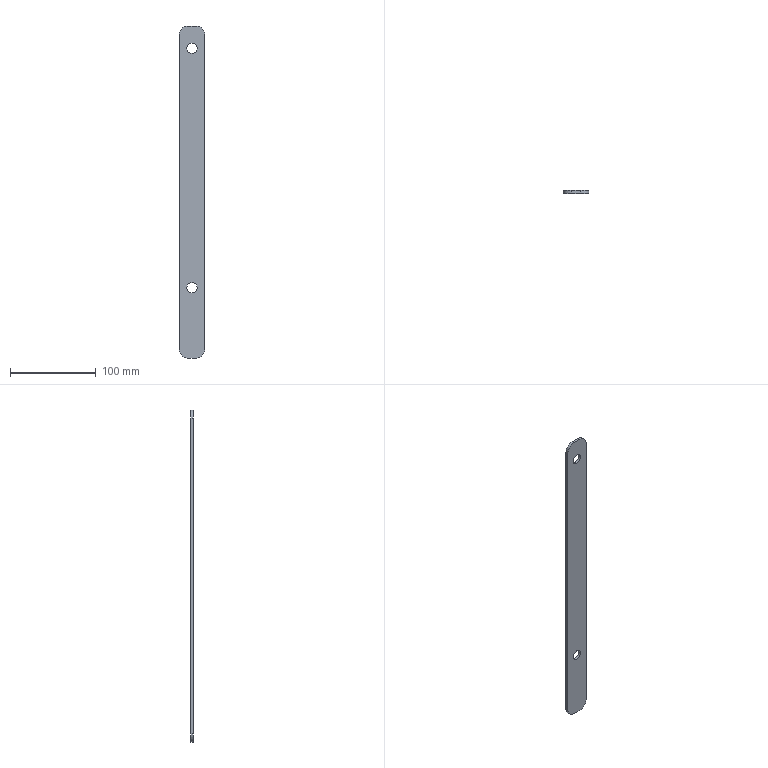Part | SolidWorks | features FlatPattern 1, SMBaseFlange 1, SheetMetal 1 | 1 solid | 14 faces | box 30 x 3.2 x 388 mm | volume 36249 mm3 | cylinder 8 | plane 6 | commonest cylinder face diameters 12 x4 20 x4
STEP:
#1=CARTESIAN_POINT('',(15.,-3.2,76.));
#2=VERTEX_POINT('',#1);
#3=CARTESIAN_POINT('',(15.,-3.2,88.));
#4=VERTEX_POINT('',#3);
#5=CARTESIAN_POINT('',(15.,-3.2,82.));
#6=DIRECTION('',(0.,1.,0.));
#7=DIRECTION('',(0.,0.,1.));
#8=AXIS2_PLACEMENT_3D('',#5,#6,#7);
#9=CIRCLE('',#8,6.);
#10=EDGE_CURVE('',#2,#4,#9,.T.);
#11=ORIENTED_EDGE('',*,*,#10,.F.);
#12=CARTESIAN_POINT('',(15.,0.,76.));
#13=VERTEX_POINT('',#12);
#14=CARTESIAN_POINT('',(15.,-3.2,76.));
#15=DIRECTION('',(0.,1.,0.));
#16=VECTOR('',#15,1000.);
#17=LINE('',#14,#16);
#18=EDGE_CURVE('',#2,#13,#17,.T.);
#19=ORIENTED_EDGE('',*,*,#18,.T.);
#20=CARTESIAN_POINT('',(15.,0.,88.));
#21=VERTEX_POINT('',#20);
#22=CARTESIAN_POINT('',(15.,0.,82.));
#23=DIRECTION('',(0.,1.,0.));
#24=DIRECTION('',(0.,0.,1.));
#25=AXIS2_PLACEMENT_3D('',#22,#23,#24);
#26=CIRCLE('',#25,6.);
#27=EDGE_CURVE('',#13,#21,#26,.T.);
#28=ORIENTED_EDGE('',*,*,#27,.T.);
#29=CARTESIAN_POINT('',(15.,-3.2,88.));
#30=DIRECTION('',(0.,1.,0.));
#31=VECTOR('',#30,1000.);
#32=LINE('',#29,#31);
#33=EDGE_CURVE('',#4,#21,#32,.T.);
#34=ORIENTED_EDGE('',*,*,#33,.F.);
#35=EDGE_LOOP('',(#11,#19,#28,#34));
#36=FACE_OUTER_BOUND('',#35,.T.);
#37=CARTESIAN_POINT('',(15.,-3.2,82.));
#38=DIRECTION('',(0.,1.,0.));
#39=DIRECTION('',(0.,0.,1.));
#40=AXIS2_PLACEMENT_3D('',#37,#38,#39);
#41=CYLINDRICAL_SURFACE('',#40,6.);
#42=ADVANCED_FACE('',(#36),#41,.F.);
#43=CARTESIAN_POINT('',(15.,-3.2,356.));
#44=VERTEX_POINT('',#43);
#45=CARTESIAN_POINT('',(15.,-3.2,368.));
#46=VERTEX_POINT('',#45);
#47=CARTESIAN_POINT('',(15.,-3.2,362.));
#48=DIRECTION('',(0.,1.,0.));
#49=DIRECTION('',(0.,0.,1.));
#50=AXIS2_PLACEMENT_3D('',#47,#48,#49);
#51=CIRCLE('',#50,6.);
#52=EDGE_CURVE('',#44,#46,#51,.T.);
#53=ORIENTED_EDGE('',*,*,#52,.F.);
#54=CARTESIAN_POINT('',(15.,0.,356.));
#55=VERTEX_POINT('',#54);
#56=CARTESIAN_POINT('',(15.,-3.2,356.));
#57=DIRECTION('',(0.,1.,0.));
#58=VECTOR('',#57,1000.);
#59=LINE('',#56,#58);
#60=EDGE_CURVE('',#44,#55,#59,.T.);
#61=ORIENTED_EDGE('',*,*,#60,.T.);
#62=CARTESIAN_POINT('',(15.,0.,368.));
#63=VERTEX_POINT('',#62);
#64=CARTESIAN_POINT('',(15.,0.,362.));
#65=DIRECTION('',(0.,1.,0.));
#66=DIRECTION('',(0.,0.,1.));
#67=AXIS2_PLACEMENT_3D('',#64,#65,#66);
#68=CIRCLE('',#67,6.);
#69=EDGE_CURVE('',#55,#63,#68,.T.);
#70=ORIENTED_EDGE('',*,*,#69,.T.);
#71=CARTESIAN_POINT('',(15.,-3.2,368.));
#72=DIRECTION('',(0.,1.,0.));
#73=VECTOR('',#72,1000.);
#74=LINE('',#71,#73);
#75=EDGE_CURVE('',#46,#63,#74,.T.);
#76=ORIENTED_EDGE('',*,*,#75,.F.);
#77=EDGE_LOOP('',(#53,#61,#70,#76));
#78=FACE_OUTER_BOUND('',#77,.T.);
#79=CARTESIAN_POINT('',(15.,-3.2,362.));
#80=DIRECTION('',(0.,1.,0.));
#81=DIRECTION('',(0.,0.,1.));
#82=AXIS2_PLACEMENT_3D('',#79,#80,#81);
#83=CYLINDRICAL_SURFACE('',#82,6.);
#84=ADVANCED_FACE('',(#78),#83,.F.);
#85=CARTESIAN_POINT('',(0.,0.,378.));
#86=VERTEX_POINT('',#85);
#87=CARTESIAN_POINT('',(10.,0.,388.));
#88=VERTEX_POINT('',#87);
#89=CARTESIAN_POINT('',(10.,0.,378.));
#90=DIRECTION('',(0.,1.,0.));
#91=DIRECTION('',(0.,0.,1.));
#92=AXIS2_PLACEMENT_3D('',#89,#90,#91);
#93=CIRCLE('',#92,10.);
#94=EDGE_CURVE('',#86,#88,#93,.T.);
#95=ORIENTED_EDGE('',*,*,#94,.F.);
#96=CARTESIAN_POINT('',(0.,-3.2,378.));
#97=VERTEX_POINT('',#96);
#98=CARTESIAN_POINT('',(0.,-3.2,378.));
#99=DIRECTION('',(0.,1.,0.));
#100=VECTOR('',#99,1000.);
#101=LINE('',#98,#100);
#102=EDGE_CURVE('',#97,#86,#101,.T.);
#103=ORIENTED_EDGE('',*,*,#102,.F.);
#104=CARTESIAN_POINT('',(10.,-3.2,388.));
#105=VERTEX_POINT('',#104);
#106=CARTESIAN_POINT('',(10.,-3.2,378.));
#107=DIRECTION('',(0.,1.,0.));
#108=DIRECTION('',(0.,0.,1.));
#109=AXIS2_PLACEMENT_3D('',#106,#107,#108);
#110=CIRCLE('',#109,10.);
#111=EDGE_CURVE('',#97,#105,#110,.T.);
#112=ORIENTED_EDGE('',*,*,#111,.T.);
#113=CARTESIAN_POINT('',(10.,-3.2,388.));
#114=DIRECTION('',(0.,1.,0.));
#115=VECTOR('',#114,1000.);
#116=LINE('',#113,#115);
#117=EDGE_CURVE('',#105,#88,#116,.T.);
#118=ORIENTED_EDGE('',*,*,#117,.T.);
#119=EDGE_LOOP('',(#95,#103,#112,#118));
#120=FACE_OUTER_BOUND('',#119,.T.);
#121=CARTESIAN_POINT('',(10.,-3.2,378.));
#122=DIRECTION('',(0.,1.,0.));
#123=DIRECTION('',(0.,0.,1.));
#124=AXIS2_PLACEMENT_3D('',#121,#122,#123);
#125=CYLINDRICAL_SURFACE('',#124,10.);
#126=ADVANCED_FACE('',(#120),#125,.T.);
#127=CARTESIAN_POINT('',(0.,0.,10.));
#128=VERTEX_POINT('',#127);
#129=CARTESIAN_POINT('',(0.,0.,10.));
#130=DIRECTION('',(0.,0.,1.));
#131=VECTOR('',#130,1000.);
#132=LINE('',#129,#131);
#133=EDGE_CURVE('',#128,#86,#132,.T.);
#134=ORIENTED_EDGE('',*,*,#133,.F.);
#135=CARTESIAN_POINT('',(0.,-3.2,10.));
#136=VERTEX_POINT('',#135);
#137=CARTESIAN_POINT('',(0.,-3.2,10.));
#138=DIRECTION('',(0.,1.,0.));
#139=VECTOR('',#138,1000.);
#140=LINE('',#137,#139);
#141=EDGE_CURVE('',#136,#128,#140,.T.);
#142=ORIENTED_EDGE('',*,*,#141,.F.);
#143=CARTESIAN_POINT('',(0.,-3.2,10.));
#144=DIRECTION('',(0.,0.,1.));
#145=VECTOR('',#144,1000.);
#146=LINE('',#143,#145);
#147=EDGE_CURVE('',#136,#97,#146,.T.);
#148=ORIENTED_EDGE('',*,*,#147,.T.);
#149=ORIENTED_EDGE('',*,*,#102,.T.);
#150=EDGE_LOOP('',(#134,#142,#148,#149));
#151=FACE_OUTER_BOUND('',#150,.T.);
#152=CARTESIAN_POINT('',(0.,-3.2,10.));
#153=DIRECTION('',(-1.,0.,0.));
#154=DIRECTION('',(0.,0.,1.));
#155=AXIS2_PLACEMENT_3D('',#152,#153,#154);
#156=PLANE('',#155);
#157=ADVANCED_FACE('',(#151),#156,.T.);
#158=CARTESIAN_POINT('',(10.,0.,0.));
#159=VERTEX_POINT('',#158);
#160=CARTESIAN_POINT('',(10.,0.,10.));
#161=DIRECTION('',(0.,1.,0.));
#162=DIRECTION('',(0.,0.,1.));
#163=AXIS2_PLACEMENT_3D('',#160,#161,#162);
#164=CIRCLE('',#163,10.);
#165=EDGE_CURVE('',#159,#128,#164,.T.);
#166=ORIENTED_EDGE('',*,*,#165,.F.);
#167=CARTESIAN_POINT('',(10.,-3.2,0.));
#168=VERTEX_POINT('',#167);
#169=CARTESIAN_POINT('',(10.,-3.2,0.));
#170=DIRECTION('',(0.,1.,0.));
#171=VECTOR('',#170,1000.);
#172=LINE('',#169,#171);
#173=EDGE_CURVE('',#168,#159,#172,.T.);
#174=ORIENTED_EDGE('',*,*,#173,.F.);
#175=CARTESIAN_POINT('',(10.,-3.2,10.));
#176=DIRECTION('',(0.,1.,0.));
#177=DIRECTION('',(0.,0.,1.));
#178=AXIS2_PLACEMENT_3D('',#175,#176,#177);
#179=CIRCLE('',#178,10.);
#180=EDGE_CURVE('',#168,#136,#179,.T.);
#181=ORIENTED_EDGE('',*,*,#180,.T.);
#182=ORIENTED_EDGE('',*,*,#141,.T.);
#183=EDGE_LOOP('',(#166,#174,#181,#182));
#184=FACE_OUTER_BOUND('',#183,.T.);
#185=CARTESIAN_POINT('',(10.,-3.2,10.));
#186=DIRECTION('',(0.,1.,0.));
#187=DIRECTION('',(0.,0.,1.));
#188=AXIS2_PLACEMENT_3D('',#185,#186,#187);
#189=CYLINDRICAL_SURFACE('',#188,10.);
#190=ADVANCED_FACE('',(#184),#189,.T.);
#191=CARTESIAN_POINT('',(20.,0.,0.));
#192=VERTEX_POINT('',#191);
#193=CARTESIAN_POINT('',(10.,0.,0.));
#194=DIRECTION('',(-1.,0.,0.));
#195=VECTOR('',#194,1000.);
#196=LINE('',#193,#195);
#197=EDGE_CURVE('',#192,#159,#196,.T.);
#198=ORIENTED_EDGE('',*,*,#197,.F.);
#199=CARTESIAN_POINT('',(20.,-3.2,0.));
#200=VERTEX_POINT('',#199);
#201=CARTESIAN_POINT('',(20.,-3.2,0.));
#202=DIRECTION('',(0.,1.,0.));
#203=VECTOR('',#202,1000.);
#204=LINE('',#201,#203);
#205=EDGE_CURVE('',#200,#192,#204,.T.);
#206=ORIENTED_EDGE('',*,*,#205,.F.);
#207=CARTESIAN_POINT('',(10.,-3.2,0.));
#208=DIRECTION('',(-1.,0.,0.));
#209=VECTOR('',#208,1000.);
#210=LINE('',#207,#209);
#211=EDGE_CURVE('',#200,#168,#210,.T.);
#212=ORIENTED_EDGE('',*,*,#211,.T.);
#213=ORIENTED_EDGE('',*,*,#173,.T.);
#214=EDGE_LOOP('',(#198,#206,#212,#213));
#215=FACE_OUTER_BOUND('',#214,.T.);
#216=CARTESIAN_POINT('',(10.,-3.2,0.));
#217=DIRECTION('',(0.,0.,-1.));
#218=DIRECTION('',(-1.,0.,0.));
#219=AXIS2_PLACEMENT_3D('',#216,#217,#218);
#220=PLANE('',#219);
#221=ADVANCED_FACE('',(#215),#220,.T.);
#222=CARTESIAN_POINT('',(30.,0.,10.));
#223=VERTEX_POINT('',#222);
#224=CARTESIAN_POINT('',(20.,0.,10.));
#225=DIRECTION('',(0.,1.,0.));
#226=DIRECTION('',(0.,0.,-1.));
#227=AXIS2_PLACEMENT_3D('',#224,#225,#226);
#228=CIRCLE('',#227,10.);
#229=EDGE_CURVE('',#223,#192,#228,.T.);
#230=ORIENTED_EDGE('',*,*,#229,.F.);
#231=CARTESIAN_POINT('',(30.,-3.2,10.));
#232=VERTEX_POINT('',#231);
#233=CARTESIAN_POINT('',(30.,-3.2,10.));
#234=DIRECTION('',(0.,1.,0.));
#235=VECTOR('',#234,1000.);
#236=LINE('',#233,#235);
#237=EDGE_CURVE('',#232,#223,#236,.T.);
#238=ORIENTED_EDGE('',*,*,#237,.F.);
#239=CARTESIAN_POINT('',(20.,-3.2,10.));
#240=DIRECTION('',(0.,1.,0.));
#241=DIRECTION('',(0.,0.,-1.));
#242=AXIS2_PLACEMENT_3D('',#239,#240,#241);
#243=CIRCLE('',#242,10.);
#244=EDGE_CURVE('',#232,#200,#243,.T.);
#245=ORIENTED_EDGE('',*,*,#244,.T.);
#246=ORIENTED_EDGE('',*,*,#205,.T.);
#247=EDGE_LOOP('',(#230,#238,#245,#246));
#248=FACE_OUTER_BOUND('',#247,.T.);
#249=CARTESIAN_POINT('',(20.,-3.2,10.));
#250=DIRECTION('',(0.,1.,0.));
#251=DIRECTION('',(0.,0.,1.));
#252=AXIS2_PLACEMENT_3D('',#249,#250,#251);
#253=CYLINDRICAL_SURFACE('',#252,10.);
#254=ADVANCED_FACE('',(#248),#253,.T.);
#255=CARTESIAN_POINT('',(30.,0.,378.));
#256=VERTEX_POINT('',#255);
#257=CARTESIAN_POINT('',(30.,0.,10.));
#258=DIRECTION('',(0.,0.,-1.));
#259=VECTOR('',#258,1000.);
#260=LINE('',#257,#259);
#261=EDGE_CURVE('',#256,#223,#260,.T.);
#262=ORIENTED_EDGE('',*,*,#261,.F.);
#263=CARTESIAN_POINT('',(30.,-3.2,378.));
#264=VERTEX_POINT('',#263);
#265=CARTESIAN_POINT('',(30.,-3.2,378.));
#266=DIRECTION('',(0.,1.,0.));
#267=VECTOR('',#266,1000.);
#268=LINE('',#265,#267);
#269=EDGE_CURVE('',#264,#256,#268,.T.);
#270=ORIENTED_EDGE('',*,*,#269,.F.);
#271=CARTESIAN_POINT('',(30.,-3.2,10.));
#272=DIRECTION('',(0.,0.,-1.));
#273=VECTOR('',#272,1000.);
#274=LINE('',#271,#273);
#275=EDGE_CURVE('',#264,#232,#274,.T.);
#276=ORIENTED_EDGE('',*,*,#275,.T.);
#277=ORIENTED_EDGE('',*,*,#237,.T.);
#278=EDGE_LOOP('',(#262,#270,#276,#277));
#279=FACE_OUTER_BOUND('',#278,.T.);
#280=CARTESIAN_POINT('',(30.,-3.2,10.));
#281=DIRECTION('',(1.,0.,0.));
#282=DIRECTION('',(0.,0.,-1.));
#283=AXIS2_PLACEMENT_3D('',#280,#281,#282);
#284=PLANE('',#283);
#285=ADVANCED_FACE('',(#279),#284,.T.);
#286=CARTESIAN_POINT('',(20.,0.,388.));
#287=VERTEX_POINT('',#286);
#288=CARTESIAN_POINT('',(20.,0.,378.));
#289=DIRECTION('',(0.,1.,0.));
#290=DIRECTION('',(0.,0.,1.));
#291=AXIS2_PLACEMENT_3D('',#288,#289,#290);
#292=CIRCLE('',#291,10.);
#293=EDGE_CURVE('',#287,#256,#292,.T.);
#294=ORIENTED_EDGE('',*,*,#293,.F.);
#295=CARTESIAN_POINT('',(20.,-3.2,388.));
#296=VERTEX_POINT('',#295);
#297=CARTESIAN_POINT('',(20.,-3.2,388.));
#298=DIRECTION('',(0.,1.,0.));
#299=VECTOR('',#298,1000.);
#300=LINE('',#297,#299);
#301=EDGE_CURVE('',#296,#287,#300,.T.);
#302=ORIENTED_EDGE('',*,*,#301,.F.);
#303=CARTESIAN_POINT('',(20.,-3.2,378.));
#304=DIRECTION('',(0.,1.,0.));
#305=DIRECTION('',(0.,0.,1.));
#306=AXIS2_PLACEMENT_3D('',#303,#304,#305);
#307=CIRCLE('',#306,10.);
#308=EDGE_CURVE('',#296,#264,#307,.T.);
#309=ORIENTED_EDGE('',*,*,#308,.T.);
#310=ORIENTED_EDGE('',*,*,#269,.T.);
#311=EDGE_LOOP('',(#294,#302,#309,#310));
#312=FACE_OUTER_BOUND('',#311,.T.);
#313=CARTESIAN_POINT('',(20.,-3.2,378.));
#314=DIRECTION('',(0.,1.,0.));
#315=DIRECTION('',(0.,0.,1.));
#316=AXIS2_PLACEMENT_3D('',#313,#314,#315);
#317=CYLINDRICAL_SURFACE('',#316,10.);
#318=ADVANCED_FACE('',(#312),#317,.T.);
#319=CARTESIAN_POINT('',(10.,0.,388.));
#320=DIRECTION('',(1.,0.,0.));
#321=VECTOR('',#320,1000.);
#322=LINE('',#319,#321);
#323=EDGE_CURVE('',#88,#287,#322,.T.);
#324=ORIENTED_EDGE('',*,*,#323,.F.);
#325=ORIENTED_EDGE('',*,*,#117,.F.);
#326=CARTESIAN_POINT('',(10.,-3.2,388.));
#327=DIRECTION('',(1.,0.,0.));
#328=VECTOR('',#327,1000.);
#329=LINE('',#326,#328);
#330=EDGE_CURVE('',#105,#296,#329,.T.);
#331=ORIENTED_EDGE('',*,*,#330,.T.);
#332=ORIENTED_EDGE('',*,*,#301,.T.);
#333=EDGE_LOOP('',(#324,#325,#331,#332));
#334=FACE_OUTER_BOUND('',#333,.T.);
#335=CARTESIAN_POINT('',(10.,-3.2,388.));
#336=DIRECTION('',(0.,0.,1.));
#337=DIRECTION('',(1.,0.,0.));
#338=AXIS2_PLACEMENT_3D('',#335,#336,#337);
#339=PLANE('',#338);
#340=ADVANCED_FACE('',(#334),#339,.T.);
#341=CARTESIAN_POINT('',(15.,-3.2,82.));
#342=DIRECTION('',(0.,1.,0.));
#343=DIRECTION('',(0.,0.,1.));
#344=AXIS2_PLACEMENT_3D('',#341,#342,#343);
#345=CIRCLE('',#344,6.);
#346=EDGE_CURVE('',#4,#2,#345,.T.);
#347=ORIENTED_EDGE('',*,*,#346,.T.);
#348=ORIENTED_EDGE('',*,*,#10,.T.);
#349=EDGE_LOOP('',(#347,#348));
#350=FACE_BOUND('',#349,.T.);
#351=CARTESIAN_POINT('',(15.,-3.2,362.));
#352=DIRECTION('',(0.,1.,0.));
#353=DIRECTION('',(0.,0.,1.));
#354=AXIS2_PLACEMENT_3D('',#351,#352,#353);
#355=CIRCLE('',#354,6.);
#356=EDGE_CURVE('',#46,#44,#355,.T.);
#357=ORIENTED_EDGE('',*,*,#356,.T.);
#358=ORIENTED_EDGE('',*,*,#52,.T.);
#359=EDGE_LOOP('',(#357,#358));
#360=FACE_BOUND('',#359,.T.);
#361=ORIENTED_EDGE('',*,*,#111,.F.);
#362=ORIENTED_EDGE('',*,*,#147,.F.);
#363=ORIENTED_EDGE('',*,*,#180,.F.);
#364=ORIENTED_EDGE('',*,*,#211,.F.);
#365=ORIENTED_EDGE('',*,*,#244,.F.);
#366=ORIENTED_EDGE('',*,*,#275,.F.);
#367=ORIENTED_EDGE('',*,*,#308,.F.);
#368=ORIENTED_EDGE('',*,*,#330,.F.);
#369=EDGE_LOOP('',(#361,#362,#363,#364,#365,#366,#367,#368));
#370=FACE_OUTER_BOUND('',#369,.T.);
#371=CARTESIAN_POINT('',(10.,-3.2,378.));
#372=DIRECTION('',(0.,1.,0.));
#373=DIRECTION('',(0.,0.,1.));
#374=AXIS2_PLACEMENT_3D('',#371,#372,#373);
#375=PLANE('',#374);
#376=ADVANCED_FACE('',(#350,#360,#370),#375,.F.);
#377=CARTESIAN_POINT('',(15.,0.,82.));
#378=DIRECTION('',(0.,1.,0.));
#379=DIRECTION('',(0.,0.,1.));
#380=AXIS2_PLACEMENT_3D('',#377,#378,#379);
#381=CIRCLE('',#380,6.);
#382=EDGE_CURVE('',#21,#13,#381,.T.);
#383=ORIENTED_EDGE('',*,*,#382,.F.);
#384=ORIENTED_EDGE('',*,*,#27,.F.);
#385=EDGE_LOOP('',(#383,#384));
#386=FACE_BOUND('',#385,.T.);
#387=CARTESIAN_POINT('',(15.,0.,362.));
#388=DIRECTION('',(0.,1.,0.));
#389=DIRECTION('',(0.,0.,1.));
#390=AXIS2_PLACEMENT_3D('',#387,#388,#389);
#391=CIRCLE('',#390,6.);
#392=EDGE_CURVE('',#63,#55,#391,.T.);
#393=ORIENTED_EDGE('',*,*,#392,.F.);
#394=ORIENTED_EDGE('',*,*,#69,.F.);
#395=EDGE_LOOP('',(#393,#394));
#396=FACE_BOUND('',#395,.T.);
#397=ORIENTED_EDGE('',*,*,#94,.T.);
#398=ORIENTED_EDGE('',*,*,#323,.T.);
#399=ORIENTED_EDGE('',*,*,#293,.T.);
#400=ORIENTED_EDGE('',*,*,#261,.T.);
#401=ORIENTED_EDGE('',*,*,#229,.T.);
#402=ORIENTED_EDGE('',*,*,#197,.T.);
#403=ORIENTED_EDGE('',*,*,#165,.T.);
#404=ORIENTED_EDGE('',*,*,#133,.T.);
#405=EDGE_LOOP('',(#397,#398,#399,#400,#401,#402,#403,#404));
#406=FACE_OUTER_BOUND('',#405,.T.);
#407=CARTESIAN_POINT('',(10.,0.,378.));
#408=DIRECTION('',(0.,1.,0.));
#409=DIRECTION('',(0.,0.,1.));
#410=AXIS2_PLACEMENT_3D('',#407,#408,#409);
#411=PLANE('',#410);
#412=ADVANCED_FACE('',(#386,#396,#406),#411,.T.);
#413=ORIENTED_EDGE('',*,*,#60,.F.);
#414=ORIENTED_EDGE('',*,*,#356,.F.);
#415=ORIENTED_EDGE('',*,*,#75,.T.);
#416=ORIENTED_EDGE('',*,*,#392,.T.);
#417=EDGE_LOOP('',(#413,#414,#415,#416));
#418=FACE_OUTER_BOUND('',#417,.T.);
#419=CARTESIAN_POINT('',(15.,-3.2,362.));
#420=DIRECTION('',(0.,1.,0.));
#421=DIRECTION('',(0.,0.,1.));
#422=AXIS2_PLACEMENT_3D('',#419,#420,#421);
#423=CYLINDRICAL_SURFACE('',#422,6.);
#424=ADVANCED_FACE('',(#418),#423,.F.);
#425=ORIENTED_EDGE('',*,*,#18,.F.);
#426=ORIENTED_EDGE('',*,*,#346,.F.);
#427=ORIENTED_EDGE('',*,*,#33,.T.);
#428=ORIENTED_EDGE('',*,*,#382,.T.);
#429=EDGE_LOOP('',(#425,#426,#427,#428));
#430=FACE_OUTER_BOUND('',#429,.T.);
#431=CARTESIAN_POINT('',(15.,-3.2,82.));
#432=DIRECTION('',(0.,1.,0.));
#433=DIRECTION('',(0.,0.,1.));
#434=AXIS2_PLACEMENT_3D('',#431,#432,#433);
#435=CYLINDRICAL_SURFACE('',#434,6.);
#436=ADVANCED_FACE('',(#430),#435,.F.);
#437=CLOSED_SHELL('',(#42,#84,#126,#157,#190,#221,#254,#285,#318,#340,#376,#412,#424,#436));
#438=MANIFOLD_SOLID_BREP('',#437);
#439=CARTESIAN_POINT('',(0.,0.,0.));
#440=DIRECTION('',(0.,0.,1.));
#441=DIRECTION('',(1.,0.,0.));
#442=AXIS2_PLACEMENT_3D('',#439,#440,#441);
#443=(LENGTH_UNIT()NAMED_UNIT(*)SI_UNIT(.MILLI.,.METRE.));
#444=UNCERTAINTY_MEASURE_WITH_UNIT(LENGTH_MEASURE(0.00001),#443,'','');
#445=(NAMED_UNIT(*)PLANE_ANGLE_UNIT()SI_UNIT($,.RADIAN.));
#446=(NAMED_UNIT(*)SI_UNIT($,.STERADIAN.)SOLID_ANGLE_UNIT());
#447=(GEOMETRIC_REPRESENTATION_CONTEXT(3)GLOBAL_UNCERTAINTY_ASSIGNED_CONTEXT((#444))GLOBAL_UNIT_ASSIGNED_CONTEXT((#443,#445,#446))REPRESENTATION_CONTEXT('',''));
#448=ADVANCED_BREP_SHAPE_REPRESENTATION('',(#438,#442),#447);